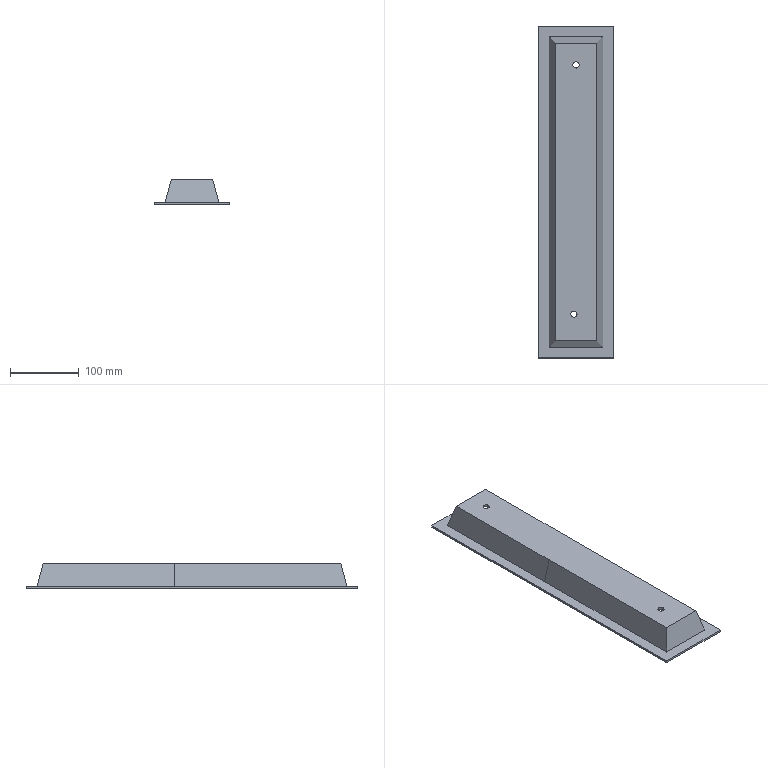Part | NX | features BREP 1 | 1 solid | 28 faces | box 110 x 481.5 x 37.13 mm | volume 237895 mm3 | plane 20 | cylinder 8 | commonest cylinder face diameters 9 x8
STEP:
#1=CARTESIAN_POINT('',(1766.215,0.,67.005));
#2=VERTEX_POINT('',#1);
#3=CARTESIAN_POINT('',(1757.07,0.,101.135));
#4=VERTEX_POINT('',#3);
#5=CARTESIAN_POINT('',(1766.215,0.,67.005));
#6=CARTESIAN_POINT('',(1757.07,0.,101.135));
#7=B_SPLINE_CURVE_WITH_KNOTS('',1,(#5,#6),.UNSPECIFIED.,.F.,.F.,(2,2),(20.364,55.698),.UNSPECIFIED.);
#8=EDGE_CURVE('',#2,#4,#7,.T.);
#9=ORIENTED_EDGE('',*,*,#8,.F.);
#10=CARTESIAN_POINT('',(1766.215,-247.843,67.005));
#11=VERTEX_POINT('',#10);
#12=CARTESIAN_POINT('',(1766.215,-123.922,67.005));
#13=DIRECTION('',(0.,1.,0.));
#14=VECTOR('',#13,1000.);
#15=LINE('',#12,#14);
#16=EDGE_CURVE('',#11,#2,#15,.T.);
#17=ORIENTED_EDGE('',*,*,#16,.F.);
#18=CARTESIAN_POINT('',(1757.07,-238.698,101.135));
#19=VERTEX_POINT('',#18);
#20=CARTESIAN_POINT('',(1761.643,-243.271,84.07));
#21=DIRECTION('',(-0.2506,0.2506,0.9351));
#22=VECTOR('',#21,1000.);
#23=LINE('',#20,#22);
#24=EDGE_CURVE('',#11,#19,#23,.T.);
#25=ORIENTED_EDGE('',*,*,#24,.T.);
#26=CARTESIAN_POINT('',(1757.07,-119.349,101.135));
#27=DIRECTION('',(0.,1.,0.));
#28=VECTOR('',#27,1000.);
#29=LINE('',#26,#28);
#30=EDGE_CURVE('',#19,#4,#29,.T.);
#31=ORIENTED_EDGE('',*,*,#30,.T.);
#32=EDGE_LOOP('',(#9,#17,#25,#31));
#33=FACE_BOUND('',#32,.T.);
#34=CARTESIAN_POINT('',(1761.643,-123.922,84.07));
#35=DIRECTION('',(0.9659,0.,0.2588));
#36=DIRECTION('',(0.2588,0.,-0.9659));
#37=AXIS2_PLACEMENT_3D('',#34,#35,#36);
#38=PLANE('',#37);
#39=ADVANCED_FACE('',(#33),#38,.F.);
#40=ORIENTED_EDGE('',*,*,#24,.F.);
#41=CARTESIAN_POINT('',(1692.529,-247.843,67.005));
#42=VERTEX_POINT('',#41);
#43=CARTESIAN_POINT('',(1729.372,-247.843,67.005));
#44=DIRECTION('',(1.,0.,0.));
#45=VECTOR('',#44,1000.);
#46=LINE('',#43,#45);
#47=EDGE_CURVE('',#42,#11,#46,.T.);
#48=ORIENTED_EDGE('',*,*,#47,.F.);
#49=CARTESIAN_POINT('',(1701.674,-238.698,101.135));
#50=VERTEX_POINT('',#49);
#51=CARTESIAN_POINT('',(1692.529,-247.843,67.005));
#52=CARTESIAN_POINT('',(1701.674,-238.698,101.135));
#53=B_SPLINE_CURVE_WITH_KNOTS('',1,(#51,#52),.UNSPECIFIED.,.F.,.F.,(2,2),(-18.249,18.249),.UNSPECIFIED.);
#54=EDGE_CURVE('',#42,#50,#53,.T.);
#55=ORIENTED_EDGE('',*,*,#54,.T.);
#56=CARTESIAN_POINT('',(1729.372,-238.698,101.135));
#57=DIRECTION('',(1.,0.,0.));
#58=VECTOR('',#57,1000.);
#59=LINE('',#56,#58);
#60=EDGE_CURVE('',#50,#19,#59,.T.);
#61=ORIENTED_EDGE('',*,*,#60,.T.);
#62=EDGE_LOOP('',(#40,#48,#55,#61));
#63=FACE_BOUND('',#62,.T.);
#64=CARTESIAN_POINT('',(1692.529,-247.843,67.005));
#65=DIRECTION('',(0.,-0.9659,0.2588));
#66=DIRECTION('',(1.,0.,0.));
#67=AXIS2_PLACEMENT_3D('',#64,#65,#66);
#68=PLANE('',#67);
#69=ADVANCED_FACE('',(#63),#68,.F.);
#70=CARTESIAN_POINT('',(1701.674,0.,101.135));
#71=VERTEX_POINT('',#70);
#72=CARTESIAN_POINT('',(1701.674,-119.349,101.135));
#73=DIRECTION('',(0.,-1.,0.));
#74=VECTOR('',#73,1000.);
#75=LINE('',#72,#74);
#76=EDGE_CURVE('',#71,#50,#75,.T.);
#77=ORIENTED_EDGE('',*,*,#76,.T.);
#78=ORIENTED_EDGE('',*,*,#54,.F.);
#79=CARTESIAN_POINT('',(1692.529,0.,67.005));
#80=VERTEX_POINT('',#79);
#81=CARTESIAN_POINT('',(1692.529,-123.922,67.005));
#82=DIRECTION('',(0.,1.,0.));
#83=VECTOR('',#82,1000.);
#84=LINE('',#81,#83);
#85=EDGE_CURVE('',#42,#80,#84,.T.);
#86=ORIENTED_EDGE('',*,*,#85,.T.);
#87=CARTESIAN_POINT('',(1692.529,0.,67.005));
#88=CARTESIAN_POINT('',(1701.674,0.,101.135));
#89=B_SPLINE_CURVE_WITH_KNOTS('',1,(#87,#88),.UNSPECIFIED.,.F.,.F.,(2,2),(20.364,55.698),.UNSPECIFIED.);
#90=EDGE_CURVE('',#80,#71,#89,.T.);
#91=ORIENTED_EDGE('',*,*,#90,.T.);
#92=EDGE_LOOP('',(#77,#78,#86,#91));
#93=FACE_BOUND('',#92,.T.);
#94=CARTESIAN_POINT('',(1697.102,-123.922,84.07));
#95=DIRECTION('',(-0.9659,0.,0.2588));
#96=DIRECTION('',(0.2588,0.,0.9659));
#97=AXIS2_PLACEMENT_3D('',#94,#95,#96);
#98=PLANE('',#97);
#99=ADVANCED_FACE('',(#93),#98,.F.);
#100=CARTESIAN_POINT('',(1692.529,197.343,67.005));
#101=VERTEX_POINT('',#100);
#102=CARTESIAN_POINT('',(1692.529,98.672,67.005));
#103=DIRECTION('',(0.,1.,0.));
#104=VECTOR('',#103,1000.);
#105=LINE('',#102,#104);
#106=EDGE_CURVE('',#80,#101,#105,.T.);
#107=ORIENTED_EDGE('',*,*,#106,.T.);
#108=CARTESIAN_POINT('',(1701.674,188.198,101.135));
#109=VERTEX_POINT('',#108);
#110=CARTESIAN_POINT('',(1692.529,197.343,67.005));
#111=CARTESIAN_POINT('',(1695.577,194.295,78.381));
#112=CARTESIAN_POINT('',(1698.626,191.246,89.758));
#113=CARTESIAN_POINT('',(1701.674,188.198,101.135));
#114=B_SPLINE_CURVE_WITH_KNOTS('',3,(#110,#111,#112,#113),.UNSPECIFIED.,.F.,.F.,(4,4),(-18.249,18.249),.UNSPECIFIED.);
#115=EDGE_CURVE('',#101,#109,#114,.T.);
#116=ORIENTED_EDGE('',*,*,#115,.T.);
#117=CARTESIAN_POINT('',(1701.674,94.099,101.135));
#118=DIRECTION('',(0.,-1.,0.));
#119=VECTOR('',#118,1000.);
#120=LINE('',#117,#119);
#121=EDGE_CURVE('',#109,#71,#120,.T.);
#122=ORIENTED_EDGE('',*,*,#121,.T.);
#123=ORIENTED_EDGE('',*,*,#90,.F.);
#124=EDGE_LOOP('',(#107,#116,#122,#123));
#125=FACE_BOUND('',#124,.T.);
#126=CARTESIAN_POINT('',(1697.102,98.672,84.07));
#127=DIRECTION('',(-0.9659,0.,0.2588));
#128=DIRECTION('',(0.2588,0.,0.9659));
#129=AXIS2_PLACEMENT_3D('',#126,#127,#128);
#130=PLANE('',#129);
#131=ADVANCED_FACE('',(#125),#130,.F.);
#132=ORIENTED_EDGE('',*,*,#115,.F.);
#133=CARTESIAN_POINT('',(1766.215,197.343,67.005));
#134=VERTEX_POINT('',#133);
#135=CARTESIAN_POINT('',(1729.372,197.343,67.005));
#136=DIRECTION('',(1.,0.,0.));
#137=VECTOR('',#136,1000.);
#138=LINE('',#135,#137);
#139=EDGE_CURVE('',#101,#134,#138,.T.);
#140=ORIENTED_EDGE('',*,*,#139,.T.);
#141=CARTESIAN_POINT('',(1757.07,188.198,101.135));
#142=VERTEX_POINT('',#141);
#143=CARTESIAN_POINT('',(1766.215,197.343,67.005));
#144=CARTESIAN_POINT('',(1757.07,188.198,101.135));
#145=B_SPLINE_CURVE_WITH_KNOTS('',1,(#143,#144),.UNSPECIFIED.,.F.,.F.,(2,2),(-18.249,18.249),.UNSPECIFIED.);
#146=EDGE_CURVE('',#134,#142,#145,.T.);
#147=ORIENTED_EDGE('',*,*,#146,.T.);
#148=CARTESIAN_POINT('',(1729.372,188.198,101.135));
#149=DIRECTION('',(-1.,0.,0.));
#150=VECTOR('',#149,1000.);
#151=LINE('',#148,#150);
#152=EDGE_CURVE('',#142,#109,#151,.T.);
#153=ORIENTED_EDGE('',*,*,#152,.T.);
#154=EDGE_LOOP('',(#132,#140,#147,#153));
#155=FACE_BOUND('',#154,.T.);
#156=CARTESIAN_POINT('',(1729.372,192.771,84.07));
#157=DIRECTION('',(0.,0.9659,0.2588));
#158=DIRECTION('',(0.,-0.2588,0.9659));
#159=AXIS2_PLACEMENT_3D('',#156,#157,#158);
#160=PLANE('',#159);
#161=ADVANCED_FACE('',(#155),#160,.F.);
#162=CARTESIAN_POINT('',(1757.07,94.099,101.135));
#163=DIRECTION('',(0.,1.,0.));
#164=VECTOR('',#163,1000.);
#165=LINE('',#162,#164);
#166=EDGE_CURVE('',#4,#142,#165,.T.);
#167=ORIENTED_EDGE('',*,*,#166,.T.);
#168=ORIENTED_EDGE('',*,*,#146,.F.);
#169=CARTESIAN_POINT('',(1766.215,98.672,67.005));
#170=DIRECTION('',(0.,1.,0.));
#171=VECTOR('',#170,1000.);
#172=LINE('',#169,#171);
#173=EDGE_CURVE('',#2,#134,#172,.T.);
#174=ORIENTED_EDGE('',*,*,#173,.F.);
#175=ORIENTED_EDGE('',*,*,#8,.T.);
#176=EDGE_LOOP('',(#167,#168,#174,#175));
#177=FACE_BOUND('',#176,.T.);
#178=CARTESIAN_POINT('',(1761.643,98.672,84.07));
#179=DIRECTION('',(0.9659,0.,0.2588));
#180=DIRECTION('',(0.2588,0.,-0.9659));
#181=AXIS2_PLACEMENT_3D('',#178,#179,#180);
#182=PLANE('',#181);
#183=ADVANCED_FACE('',(#177),#182,.F.);
#184=CARTESIAN_POINT('',(1730.872,-202.5,101.135));
#185=VERTEX_POINT('',#184);
#186=CARTESIAN_POINT('',(1726.372,-198.,101.135));
#187=VERTEX_POINT('',#186);
#188=CARTESIAN_POINT('',(1726.372,-202.5,101.135));
#189=DIRECTION('',(0.,0.,1.));
#190=DIRECTION('',(1.,0.,0.));
#191=AXIS2_PLACEMENT_3D('',#188,#189,#190);
#192=CIRCLE('',#191,4.5);
#193=EDGE_CURVE('',#185,#187,#192,.T.);
#194=ORIENTED_EDGE('',*,*,#193,.T.);
#195=CARTESIAN_POINT('',(1721.872,-202.5,101.135));
#196=VERTEX_POINT('',#195);
#197=CARTESIAN_POINT('',(1726.372,-202.5,101.135));
#198=DIRECTION('',(0.,0.,1.));
#199=DIRECTION('',(1.,0.,0.));
#200=AXIS2_PLACEMENT_3D('',#197,#198,#199);
#201=CIRCLE('',#200,4.5);
#202=EDGE_CURVE('',#187,#196,#201,.T.);
#203=ORIENTED_EDGE('',*,*,#202,.T.);
#204=CARTESIAN_POINT('',(1726.372,-207.,101.135));
#205=VERTEX_POINT('',#204);
#206=CARTESIAN_POINT('',(1726.372,-202.5,101.135));
#207=DIRECTION('',(0.,0.,1.));
#208=DIRECTION('',(1.,0.,0.));
#209=AXIS2_PLACEMENT_3D('',#206,#207,#208);
#210=CIRCLE('',#209,4.5);
#211=EDGE_CURVE('',#196,#205,#210,.T.);
#212=ORIENTED_EDGE('',*,*,#211,.T.);
#213=CARTESIAN_POINT('',(1726.372,-202.5,101.135));
#214=DIRECTION('',(0.,0.,1.));
#215=DIRECTION('',(1.,0.,0.));
#216=AXIS2_PLACEMENT_3D('',#213,#214,#215);
#217=CIRCLE('',#216,4.5);
#218=EDGE_CURVE('',#205,#185,#217,.T.);
#219=ORIENTED_EDGE('',*,*,#218,.T.);
#220=EDGE_LOOP('',(#194,#203,#212,#219));
#221=FACE_BOUND('',#220,.T.);
#222=CARTESIAN_POINT('',(1733.872,159.,101.135));
#223=VERTEX_POINT('',#222);
#224=CARTESIAN_POINT('',(1729.372,163.5,101.135));
#225=VERTEX_POINT('',#224);
#226=CARTESIAN_POINT('',(1729.372,159.,101.135));
#227=DIRECTION('',(0.,0.,1.));
#228=DIRECTION('',(1.,0.,0.));
#229=AXIS2_PLACEMENT_3D('',#226,#227,#228);
#230=CIRCLE('',#229,4.5);
#231=EDGE_CURVE('',#223,#225,#230,.T.);
#232=ORIENTED_EDGE('',*,*,#231,.T.);
#233=CARTESIAN_POINT('',(1724.872,159.,101.135));
#234=VERTEX_POINT('',#233);
#235=CARTESIAN_POINT('',(1729.372,159.,101.135));
#236=DIRECTION('',(0.,0.,1.));
#237=DIRECTION('',(1.,0.,0.));
#238=AXIS2_PLACEMENT_3D('',#235,#236,#237);
#239=CIRCLE('',#238,4.5);
#240=EDGE_CURVE('',#225,#234,#239,.T.);
#241=ORIENTED_EDGE('',*,*,#240,.T.);
#242=CARTESIAN_POINT('',(1729.372,154.5,101.135));
#243=VERTEX_POINT('',#242);
#244=CARTESIAN_POINT('',(1729.372,159.,101.135));
#245=DIRECTION('',(0.,0.,1.));
#246=DIRECTION('',(1.,0.,0.));
#247=AXIS2_PLACEMENT_3D('',#244,#245,#246);
#248=CIRCLE('',#247,4.5);
#249=EDGE_CURVE('',#234,#243,#248,.T.);
#250=ORIENTED_EDGE('',*,*,#249,.T.);
#251=CARTESIAN_POINT('',(1729.372,159.,101.135));
#252=DIRECTION('',(0.,0.,1.));
#253=DIRECTION('',(1.,0.,0.));
#254=AXIS2_PLACEMENT_3D('',#251,#252,#253);
#255=CIRCLE('',#254,4.5);
#256=EDGE_CURVE('',#243,#223,#255,.T.);
#257=ORIENTED_EDGE('',*,*,#256,.T.);
#258=EDGE_LOOP('',(#232,#241,#250,#257));
#259=FACE_BOUND('',#258,.T.);
#260=ORIENTED_EDGE('',*,*,#166,.F.);
#261=ORIENTED_EDGE('',*,*,#30,.F.);
#262=ORIENTED_EDGE('',*,*,#60,.F.);
#263=ORIENTED_EDGE('',*,*,#76,.F.);
#264=ORIENTED_EDGE('',*,*,#121,.F.);
#265=ORIENTED_EDGE('',*,*,#152,.F.);
#266=EDGE_LOOP('',(#260,#261,#262,#263,#264,#265));
#267=FACE_BOUND('',#266,.T.);
#268=CARTESIAN_POINT('',(450.,0.,101.135));
#269=DIRECTION('',(0.,0.,1.));
#270=DIRECTION('',(1.,0.,0.));
#271=AXIS2_PLACEMENT_3D('',#268,#269,#270);
#272=PLANE('',#271);
#273=ADVANCED_FACE('',(#221,#259,#267),#272,.F.);
#274=ORIENTED_EDGE('',*,*,#173,.T.);
#275=ORIENTED_EDGE('',*,*,#139,.F.);
#276=ORIENTED_EDGE('',*,*,#106,.F.);
#277=ORIENTED_EDGE('',*,*,#85,.F.);
#278=ORIENTED_EDGE('',*,*,#47,.T.);
#279=ORIENTED_EDGE('',*,*,#16,.T.);
#280=EDGE_LOOP('',(#274,#275,#276,#277,#278,#279));
#281=FACE_BOUND('',#280,.T.);
#282=CARTESIAN_POINT('',(1674.372,215.5,67.005));
#283=VERTEX_POINT('',#282);
#284=CARTESIAN_POINT('',(1784.372,215.5,67.005));
#285=VERTEX_POINT('',#284);
#286=CARTESIAN_POINT('',(1729.372,215.5,67.005));
#287=DIRECTION('',(1.,0.,0.));
#288=VECTOR('',#287,1000.);
#289=LINE('',#286,#288);
#290=EDGE_CURVE('',#283,#285,#289,.T.);
#291=ORIENTED_EDGE('',*,*,#290,.T.);
#292=CARTESIAN_POINT('',(1784.372,-266.,67.005));
#293=VERTEX_POINT('',#292);
#294=CARTESIAN_POINT('',(1784.372,-25.25,67.005));
#295=DIRECTION('',(0.,1.,0.));
#296=VECTOR('',#295,1000.);
#297=LINE('',#294,#296);
#298=EDGE_CURVE('',#293,#285,#297,.T.);
#299=ORIENTED_EDGE('',*,*,#298,.F.);
#300=CARTESIAN_POINT('',(1674.372,-266.,67.005));
#301=VERTEX_POINT('',#300);
#302=CARTESIAN_POINT('',(1729.372,-266.,67.005));
#303=DIRECTION('',(1.,0.,0.));
#304=VECTOR('',#303,1000.);
#305=LINE('',#302,#304);
#306=EDGE_CURVE('',#301,#293,#305,.T.);
#307=ORIENTED_EDGE('',*,*,#306,.F.);
#308=CARTESIAN_POINT('',(1674.372,-25.25,67.005));
#309=DIRECTION('',(0.,1.,0.));
#310=VECTOR('',#309,1000.);
#311=LINE('',#308,#310);
#312=EDGE_CURVE('',#301,#283,#311,.T.);
#313=ORIENTED_EDGE('',*,*,#312,.T.);
#314=EDGE_LOOP('',(#291,#299,#307,#313));
#315=FACE_BOUND('',#314,.T.);
#316=CARTESIAN_POINT('',(450.,0.,67.005));
#317=DIRECTION('',(0.,0.,1.));
#318=DIRECTION('',(1.,0.,0.));
#319=AXIS2_PLACEMENT_3D('',#316,#317,#318);
#320=PLANE('',#319);
#321=ADVANCED_FACE('',(#281,#315),#320,.F.);
#322=ORIENTED_EDGE('',*,*,#193,.F.);
#323=CARTESIAN_POINT('',(1730.872,-202.5,104.135));
#324=VERTEX_POINT('',#323);
#325=CARTESIAN_POINT('',(1730.872,-202.5,104.135));
#326=DIRECTION('',(0.,0.,1.));
#327=VECTOR('',#326,1000.);
#328=LINE('',#325,#327);
#329=EDGE_CURVE('',#185,#324,#328,.T.);
#330=ORIENTED_EDGE('',*,*,#329,.T.);
#331=CARTESIAN_POINT('',(1726.372,-198.,104.135));
#332=VERTEX_POINT('',#331);
#333=CARTESIAN_POINT('',(1726.372,-202.5,104.135));
#334=DIRECTION('',(0.,0.,1.));
#335=DIRECTION('',(1.,0.,0.));
#336=AXIS2_PLACEMENT_3D('',#333,#334,#335);
#337=CIRCLE('',#336,4.5);
#338=EDGE_CURVE('',#324,#332,#337,.T.);
#339=ORIENTED_EDGE('',*,*,#338,.T.);
#340=CARTESIAN_POINT('',(1726.372,-198.,104.135));
#341=DIRECTION('',(0.,0.,1.));
#342=VECTOR('',#341,1000.);
#343=LINE('',#340,#342);
#344=EDGE_CURVE('',#187,#332,#343,.T.);
#345=ORIENTED_EDGE('',*,*,#344,.F.);
#346=EDGE_LOOP('',(#322,#330,#339,#345));
#347=FACE_BOUND('',#346,.T.);
#348=CARTESIAN_POINT('',(1726.372,-202.5,104.135));
#349=DIRECTION('',(0.,0.,1.));
#350=DIRECTION('',(0.,-1.,0.));
#351=AXIS2_PLACEMENT_3D('',#348,#349,#350);
#352=CYLINDRICAL_SURFACE('',#351,4.5);
#353=ADVANCED_FACE('',(#347),#352,.F.);
#354=CARTESIAN_POINT('',(1721.872,-202.5,104.135));
#355=VERTEX_POINT('',#354);
#356=CARTESIAN_POINT('',(1726.372,-202.5,104.135));
#357=DIRECTION('',(0.,0.,1.));
#358=DIRECTION('',(1.,0.,0.));
#359=AXIS2_PLACEMENT_3D('',#356,#357,#358);
#360=CIRCLE('',#359,4.5);
#361=EDGE_CURVE('',#332,#355,#360,.T.);
#362=ORIENTED_EDGE('',*,*,#361,.T.);
#363=CARTESIAN_POINT('',(1721.872,-202.5,104.135));
#364=DIRECTION('',(0.,0.,1.));
#365=VECTOR('',#364,1000.);
#366=LINE('',#363,#365);
#367=EDGE_CURVE('',#196,#355,#366,.T.);
#368=ORIENTED_EDGE('',*,*,#367,.F.);
#369=ORIENTED_EDGE('',*,*,#202,.F.);
#370=ORIENTED_EDGE('',*,*,#344,.T.);
#371=EDGE_LOOP('',(#362,#368,#369,#370));
#372=FACE_BOUND('',#371,.T.);
#373=CARTESIAN_POINT('',(1726.372,-202.5,104.135));
#374=DIRECTION('',(0.,0.,1.));
#375=DIRECTION('',(0.,1.,0.));
#376=AXIS2_PLACEMENT_3D('',#373,#374,#375);
#377=CYLINDRICAL_SURFACE('',#376,4.5);
#378=ADVANCED_FACE('',(#372),#377,.F.);
#379=ORIENTED_EDGE('',*,*,#211,.F.);
#380=ORIENTED_EDGE('',*,*,#367,.T.);
#381=CARTESIAN_POINT('',(1726.372,-207.,104.135));
#382=VERTEX_POINT('',#381);
#383=CARTESIAN_POINT('',(1726.372,-202.5,104.135));
#384=DIRECTION('',(0.,0.,1.));
#385=DIRECTION('',(1.,0.,0.));
#386=AXIS2_PLACEMENT_3D('',#383,#384,#385);
#387=CIRCLE('',#386,4.5);
#388=EDGE_CURVE('',#355,#382,#387,.T.);
#389=ORIENTED_EDGE('',*,*,#388,.T.);
#390=CARTESIAN_POINT('',(1726.372,-207.,104.135));
#391=DIRECTION('',(0.,0.,1.));
#392=VECTOR('',#391,1000.);
#393=LINE('',#390,#392);
#394=EDGE_CURVE('',#205,#382,#393,.T.);
#395=ORIENTED_EDGE('',*,*,#394,.F.);
#396=EDGE_LOOP('',(#379,#380,#389,#395));
#397=FACE_BOUND('',#396,.T.);
#398=CARTESIAN_POINT('',(1726.372,-202.5,104.135));
#399=DIRECTION('',(0.,0.,1.));
#400=DIRECTION('',(0.,1.,0.));
#401=AXIS2_PLACEMENT_3D('',#398,#399,#400);
#402=CYLINDRICAL_SURFACE('',#401,4.5);
#403=ADVANCED_FACE('',(#397),#402,.F.);
#404=CARTESIAN_POINT('',(1726.372,-202.5,104.135));
#405=DIRECTION('',(0.,0.,1.));
#406=DIRECTION('',(1.,0.,0.));
#407=AXIS2_PLACEMENT_3D('',#404,#405,#406);
#408=CIRCLE('',#407,4.5);
#409=EDGE_CURVE('',#382,#324,#408,.T.);
#410=ORIENTED_EDGE('',*,*,#409,.T.);
#411=ORIENTED_EDGE('',*,*,#329,.F.);
#412=ORIENTED_EDGE('',*,*,#218,.F.);
#413=ORIENTED_EDGE('',*,*,#394,.T.);
#414=EDGE_LOOP('',(#410,#411,#412,#413));
#415=FACE_BOUND('',#414,.T.);
#416=CARTESIAN_POINT('',(1726.372,-202.5,104.135));
#417=DIRECTION('',(0.,0.,1.));
#418=DIRECTION('',(0.,-1.,0.));
#419=AXIS2_PLACEMENT_3D('',#416,#417,#418);
#420=CYLINDRICAL_SURFACE('',#419,4.5);
#421=ADVANCED_FACE('',(#415),#420,.F.);
#422=ORIENTED_EDGE('',*,*,#231,.F.);
#423=CARTESIAN_POINT('',(1733.872,159.,104.135));
#424=VERTEX_POINT('',#423);
#425=CARTESIAN_POINT('',(1733.872,159.,104.135));
#426=DIRECTION('',(0.,0.,1.));
#427=VECTOR('',#426,1000.);
#428=LINE('',#425,#427);
#429=EDGE_CURVE('',#223,#424,#428,.T.);
#430=ORIENTED_EDGE('',*,*,#429,.T.);
#431=CARTESIAN_POINT('',(1729.372,163.5,104.135));
#432=VERTEX_POINT('',#431);
#433=CARTESIAN_POINT('',(1729.372,159.,104.135));
#434=DIRECTION('',(0.,0.,1.));
#435=DIRECTION('',(1.,0.,0.));
#436=AXIS2_PLACEMENT_3D('',#433,#434,#435);
#437=CIRCLE('',#436,4.5);
#438=EDGE_CURVE('',#424,#432,#437,.T.);
#439=ORIENTED_EDGE('',*,*,#438,.T.);
#440=CARTESIAN_POINT('',(1729.372,163.5,104.135));
#441=DIRECTION('',(0.,0.,1.));
#442=VECTOR('',#441,1000.);
#443=LINE('',#440,#442);
#444=EDGE_CURVE('',#225,#432,#443,.T.);
#445=ORIENTED_EDGE('',*,*,#444,.F.);
#446=EDGE_LOOP('',(#422,#430,#439,#445));
#447=FACE_BOUND('',#446,.T.);
#448=CARTESIAN_POINT('',(1729.372,159.,104.135));
#449=DIRECTION('',(0.,0.,1.));
#450=DIRECTION('',(0.,-1.,0.));
#451=AXIS2_PLACEMENT_3D('',#448,#449,#450);
#452=CYLINDRICAL_SURFACE('',#451,4.5);
#453=ADVANCED_FACE('',(#447),#452,.F.);
#454=CARTESIAN_POINT('',(1724.872,159.,104.135));
#455=VERTEX_POINT('',#454);
#456=CARTESIAN_POINT('',(1729.372,159.,104.135));
#457=DIRECTION('',(0.,0.,1.));
#458=DIRECTION('',(1.,0.,0.));
#459=AXIS2_PLACEMENT_3D('',#456,#457,#458);
#460=CIRCLE('',#459,4.5);
#461=EDGE_CURVE('',#432,#455,#460,.T.);
#462=ORIENTED_EDGE('',*,*,#461,.T.);
#463=CARTESIAN_POINT('',(1724.872,159.,104.135));
#464=DIRECTION('',(0.,0.,1.));
#465=VECTOR('',#464,1000.);
#466=LINE('',#463,#465);
#467=EDGE_CURVE('',#234,#455,#466,.T.);
#468=ORIENTED_EDGE('',*,*,#467,.F.);
#469=ORIENTED_EDGE('',*,*,#240,.F.);
#470=ORIENTED_EDGE('',*,*,#444,.T.);
#471=EDGE_LOOP('',(#462,#468,#469,#470));
#472=FACE_BOUND('',#471,.T.);
#473=CARTESIAN_POINT('',(1729.372,159.,104.135));
#474=DIRECTION('',(0.,0.,1.));
#475=DIRECTION('',(0.,1.,0.));
#476=AXIS2_PLACEMENT_3D('',#473,#474,#475);
#477=CYLINDRICAL_SURFACE('',#476,4.5);
#478=ADVANCED_FACE('',(#472),#477,.F.);
#479=ORIENTED_EDGE('',*,*,#249,.F.);
#480=ORIENTED_EDGE('',*,*,#467,.T.);
#481=CARTESIAN_POINT('',(1729.372,154.5,104.135));
#482=VERTEX_POINT('',#481);
#483=CARTESIAN_POINT('',(1729.372,159.,104.135));
#484=DIRECTION('',(0.,0.,1.));
#485=DIRECTION('',(1.,0.,0.));
#486=AXIS2_PLACEMENT_3D('',#483,#484,#485);
#487=CIRCLE('',#486,4.5);
#488=EDGE_CURVE('',#455,#482,#487,.T.);
#489=ORIENTED_EDGE('',*,*,#488,.T.);
#490=CARTESIAN_POINT('',(1729.372,154.5,104.135));
#491=DIRECTION('',(0.,0.,1.));
#492=VECTOR('',#491,1000.);
#493=LINE('',#490,#492);
#494=EDGE_CURVE('',#243,#482,#493,.T.);
#495=ORIENTED_EDGE('',*,*,#494,.F.);
#496=EDGE_LOOP('',(#479,#480,#489,#495));
#497=FACE_BOUND('',#496,.T.);
#498=CARTESIAN_POINT('',(1729.372,159.,104.135));
#499=DIRECTION('',(0.,0.,1.));
#500=DIRECTION('',(0.,1.,0.));
#501=AXIS2_PLACEMENT_3D('',#498,#499,#500);
#502=CYLINDRICAL_SURFACE('',#501,4.5);
#503=ADVANCED_FACE('',(#497),#502,.F.);
#504=CARTESIAN_POINT('',(1729.372,159.,104.135));
#505=DIRECTION('',(0.,0.,1.));
#506=DIRECTION('',(1.,0.,0.));
#507=AXIS2_PLACEMENT_3D('',#504,#505,#506);
#508=CIRCLE('',#507,4.5);
#509=EDGE_CURVE('',#482,#424,#508,.T.);
#510=ORIENTED_EDGE('',*,*,#509,.T.);
#511=ORIENTED_EDGE('',*,*,#429,.F.);
#512=ORIENTED_EDGE('',*,*,#256,.F.);
#513=ORIENTED_EDGE('',*,*,#494,.T.);
#514=EDGE_LOOP('',(#510,#511,#512,#513));
#515=FACE_BOUND('',#514,.T.);
#516=CARTESIAN_POINT('',(1729.372,159.,104.135));
#517=DIRECTION('',(0.,0.,1.));
#518=DIRECTION('',(0.,-1.,0.));
#519=AXIS2_PLACEMENT_3D('',#516,#517,#518);
#520=CYLINDRICAL_SURFACE('',#519,4.5);
#521=ADVANCED_FACE('',(#515),#520,.F.);
#522=CARTESIAN_POINT('',(1768.517,0.,70.005));
#523=VERTEX_POINT('',#522);
#524=CARTESIAN_POINT('',(1759.372,0.,104.135));
#525=VERTEX_POINT('',#524);
#526=CARTESIAN_POINT('',(1768.517,0.,70.005));
#527=CARTESIAN_POINT('',(1759.372,0.,104.135));
#528=B_SPLINE_CURVE_WITH_KNOTS('',1,(#526,#527),.UNSPECIFIED.,.F.,.F.,(2,2),(22.666,58.),.UNSPECIFIED.);
#529=EDGE_CURVE('',#523,#525,#528,.T.);
#530=ORIENTED_EDGE('',*,*,#529,.F.);
#531=CARTESIAN_POINT('',(1768.517,199.645,70.005));
#532=VERTEX_POINT('',#531);
#533=CARTESIAN_POINT('',(1768.517,99.823,70.005));
#534=DIRECTION('',(0.,1.,0.));
#535=VECTOR('',#534,1000.);
#536=LINE('',#533,#535);
#537=EDGE_CURVE('',#523,#532,#536,.T.);
#538=ORIENTED_EDGE('',*,*,#537,.T.);
#539=CARTESIAN_POINT('',(1759.372,190.5,104.135));
#540=VERTEX_POINT('',#539);
#541=CARTESIAN_POINT('',(1768.517,199.645,70.005));
#542=CARTESIAN_POINT('',(1759.372,190.5,104.135));
#543=B_SPLINE_CURVE_WITH_KNOTS('',1,(#541,#542),.UNSPECIFIED.,.F.,.F.,(2,2),(-18.249,18.249),.UNSPECIFIED.);
#544=EDGE_CURVE('',#532,#540,#543,.T.);
#545=ORIENTED_EDGE('',*,*,#544,.T.);
#546=CARTESIAN_POINT('',(1759.372,95.25,104.135));
#547=DIRECTION('',(0.,1.,0.));
#548=VECTOR('',#547,1000.);
#549=LINE('',#546,#548);
#550=EDGE_CURVE('',#525,#540,#549,.T.);
#551=ORIENTED_EDGE('',*,*,#550,.F.);
#552=EDGE_LOOP('',(#530,#538,#545,#551));
#553=FACE_BOUND('',#552,.T.);
#554=CARTESIAN_POINT('',(1766.878,-50.5,76.123));
#555=DIRECTION('',(0.9659,0.,0.2588));
#556=DIRECTION('',(0.2588,0.,-0.9659));
#557=AXIS2_PLACEMENT_3D('',#554,#555,#556);
#558=PLANE('',#557);
#559=ADVANCED_FACE('',(#553),#558,.T.);
#560=CARTESIAN_POINT('',(1759.372,-241.,104.135));
#561=VERTEX_POINT('',#560);
#562=CARTESIAN_POINT('',(1759.372,-120.5,104.135));
#563=DIRECTION('',(0.,1.,0.));
#564=VECTOR('',#563,1000.);
#565=LINE('',#562,#564);
#566=EDGE_CURVE('',#561,#525,#565,.T.);
#567=ORIENTED_EDGE('',*,*,#566,.F.);
#568=CARTESIAN_POINT('',(1768.517,-250.145,70.005));
#569=VERTEX_POINT('',#568);
#570=CARTESIAN_POINT('',(1768.517,-250.145,70.005));
#571=CARTESIAN_POINT('',(1759.372,-241.,104.135));
#572=B_SPLINE_CURVE_WITH_KNOTS('',1,(#570,#571),.UNSPECIFIED.,.F.,.F.,(2,2),(-18.249,18.249),.UNSPECIFIED.);
#573=EDGE_CURVE('',#569,#561,#572,.T.);
#574=ORIENTED_EDGE('',*,*,#573,.F.);
#575=CARTESIAN_POINT('',(1768.517,-125.073,70.005));
#576=DIRECTION('',(0.,1.,0.));
#577=VECTOR('',#576,1000.);
#578=LINE('',#575,#577);
#579=EDGE_CURVE('',#569,#523,#578,.T.);
#580=ORIENTED_EDGE('',*,*,#579,.T.);
#581=ORIENTED_EDGE('',*,*,#529,.T.);
#582=EDGE_LOOP('',(#567,#574,#580,#581));
#583=FACE_BOUND('',#582,.T.);
#584=CARTESIAN_POINT('',(1766.878,0.000003927,76.123));
#585=DIRECTION('',(0.9659,0.,0.2588));
#586=DIRECTION('',(0.2588,0.,-0.9659));
#587=AXIS2_PLACEMENT_3D('',#584,#585,#586);
#588=PLANE('',#587);
#589=ADVANCED_FACE('',(#583),#588,.T.);
#590=CARTESIAN_POINT('',(1674.372,215.5,70.005));
#591=VERTEX_POINT('',#590);
#592=CARTESIAN_POINT('',(1784.372,215.5,70.005));
#593=VERTEX_POINT('',#592);
#594=CARTESIAN_POINT('',(1729.372,215.5,70.005));
#595=DIRECTION('',(1.,0.,0.));
#596=VECTOR('',#595,1000.);
#597=LINE('',#594,#596);
#598=EDGE_CURVE('',#591,#593,#597,.T.);
#599=ORIENTED_EDGE('',*,*,#598,.T.);
#600=CARTESIAN_POINT('',(1784.372,215.5,68.505));
#601=DIRECTION('',(0.,0.,-1.));
#602=VECTOR('',#601,1000.);
#603=LINE('',#600,#602);
#604=EDGE_CURVE('',#593,#285,#603,.T.);
#605=ORIENTED_EDGE('',*,*,#604,.T.);
#606=ORIENTED_EDGE('',*,*,#290,.F.);
#607=CARTESIAN_POINT('',(1674.372,215.5,68.505));
#608=DIRECTION('',(0.,0.,-1.));
#609=VECTOR('',#608,1000.);
#610=LINE('',#607,#609);
#611=EDGE_CURVE('',#591,#283,#610,.T.);
#612=ORIENTED_EDGE('',*,*,#611,.F.);
#613=EDGE_LOOP('',(#599,#605,#606,#612));
#614=FACE_BOUND('',#613,.T.);
#615=CARTESIAN_POINT('',(1729.372,215.5,70.005));
#616=DIRECTION('',(0.,1.,0.));
#617=DIRECTION('',(1.,0.,0.));
#618=AXIS2_PLACEMENT_3D('',#615,#616,#617);
#619=PLANE('',#618);
#620=ADVANCED_FACE('',(#614),#619,.T.);
#621=CARTESIAN_POINT('',(1784.372,-266.,70.005));
#622=VERTEX_POINT('',#621);
#623=CARTESIAN_POINT('',(1784.372,-25.25,70.005));
#624=DIRECTION('',(0.,-1.,0.));
#625=VECTOR('',#624,1000.);
#626=LINE('',#623,#625);
#627=EDGE_CURVE('',#593,#622,#626,.T.);
#628=ORIENTED_EDGE('',*,*,#627,.T.);
#629=CARTESIAN_POINT('',(1784.372,-266.,68.505));
#630=DIRECTION('',(0.,0.,-1.));
#631=VECTOR('',#630,1000.);
#632=LINE('',#629,#631);
#633=EDGE_CURVE('',#622,#293,#632,.T.);
#634=ORIENTED_EDGE('',*,*,#633,.T.);
#635=ORIENTED_EDGE('',*,*,#298,.T.);
#636=ORIENTED_EDGE('',*,*,#604,.F.);
#637=EDGE_LOOP('',(#628,#634,#635,#636));
#638=FACE_BOUND('',#637,.T.);
#639=CARTESIAN_POINT('',(1784.372,-25.25,70.005));
#640=DIRECTION('',(-1.,0.,0.));
#641=DIRECTION('',(0.,0.,-1.));
#642=AXIS2_PLACEMENT_3D('',#639,#640,#641);
#643=PLANE('',#642);
#644=ADVANCED_FACE('',(#638),#643,.F.);
#645=CARTESIAN_POINT('',(1674.372,-266.,70.005));
#646=VERTEX_POINT('',#645);
#647=CARTESIAN_POINT('',(1729.372,-266.,70.005));
#648=DIRECTION('',(1.,0.,0.));
#649=VECTOR('',#648,1000.);
#650=LINE('',#647,#649);
#651=EDGE_CURVE('',#646,#622,#650,.T.);
#652=ORIENTED_EDGE('',*,*,#651,.F.);
#653=CARTESIAN_POINT('',(1674.372,-266.,68.505));
#654=DIRECTION('',(0.,0.,-1.));
#655=VECTOR('',#654,1000.);
#656=LINE('',#653,#655);
#657=EDGE_CURVE('',#646,#301,#656,.T.);
#658=ORIENTED_EDGE('',*,*,#657,.T.);
#659=ORIENTED_EDGE('',*,*,#306,.T.);
#660=ORIENTED_EDGE('',*,*,#633,.F.);
#661=EDGE_LOOP('',(#652,#658,#659,#660));
#662=FACE_BOUND('',#661,.T.);
#663=CARTESIAN_POINT('',(1729.372,-266.,70.005));
#664=DIRECTION('',(0.,1.,0.));
#665=DIRECTION('',(1.,0.,0.));
#666=AXIS2_PLACEMENT_3D('',#663,#664,#665);
#667=PLANE('',#666);
#668=ADVANCED_FACE('',(#662),#667,.F.);
#669=ORIENTED_EDGE('',*,*,#611,.T.);
#670=ORIENTED_EDGE('',*,*,#312,.F.);
#671=ORIENTED_EDGE('',*,*,#657,.F.);
#672=CARTESIAN_POINT('',(1674.372,-25.25,70.005));
#673=DIRECTION('',(0.,1.,0.));
#674=VECTOR('',#673,1000.);
#675=LINE('',#672,#674);
#676=EDGE_CURVE('',#646,#591,#675,.T.);
#677=ORIENTED_EDGE('',*,*,#676,.T.);
#678=EDGE_LOOP('',(#669,#670,#671,#677));
#679=FACE_BOUND('',#678,.T.);
#680=CARTESIAN_POINT('',(1674.372,-25.25,70.005));
#681=DIRECTION('',(1.,0.,0.));
#682=DIRECTION('',(0.,0.,-1.));
#683=AXIS2_PLACEMENT_3D('',#680,#681,#682);
#684=PLANE('',#683);
#685=ADVANCED_FACE('',(#679),#684,.F.);
#686=CARTESIAN_POINT('',(1699.372,190.5,104.135));
#687=VERTEX_POINT('',#686);
#688=CARTESIAN_POINT('',(1729.372,190.5,104.135));
#689=DIRECTION('',(-1.,0.,0.));
#690=VECTOR('',#689,1000.);
#691=LINE('',#688,#690);
#692=EDGE_CURVE('',#540,#687,#691,.T.);
#693=ORIENTED_EDGE('',*,*,#692,.F.);
#694=ORIENTED_EDGE('',*,*,#544,.F.);
#695=CARTESIAN_POINT('',(1690.227,199.645,70.005));
#696=VERTEX_POINT('',#695);
#697=CARTESIAN_POINT('',(1729.372,199.645,70.005));
#698=DIRECTION('',(-1.,0.,0.));
#699=VECTOR('',#698,1000.);
#700=LINE('',#697,#699);
#701=EDGE_CURVE('',#532,#696,#700,.T.);
#702=ORIENTED_EDGE('',*,*,#701,.T.);
#703=CARTESIAN_POINT('',(1690.227,199.645,70.005));
#704=CARTESIAN_POINT('',(1699.372,190.5,104.135));
#705=B_SPLINE_CURVE_WITH_KNOTS('',1,(#703,#704),.UNSPECIFIED.,.F.,.F.,(2,2),(-18.249,18.249),.UNSPECIFIED.);
#706=EDGE_CURVE('',#696,#687,#705,.T.);
#707=ORIENTED_EDGE('',*,*,#706,.T.);
#708=EDGE_LOOP('',(#693,#694,#702,#707));
#709=FACE_BOUND('',#708,.T.);
#710=CARTESIAN_POINT('',(1729.372,198.006,76.123));
#711=DIRECTION('',(0.,0.9659,0.2588));
#712=DIRECTION('',(0.,-0.2588,0.9659));
#713=AXIS2_PLACEMENT_3D('',#710,#711,#712);
#714=PLANE('',#713);
#715=ADVANCED_FACE('',(#709),#714,.T.);
#716=ORIENTED_EDGE('',*,*,#409,.F.);
#717=ORIENTED_EDGE('',*,*,#388,.F.);
#718=ORIENTED_EDGE('',*,*,#361,.F.);
#719=ORIENTED_EDGE('',*,*,#338,.F.);
#720=EDGE_LOOP('',(#716,#717,#718,#719));
#721=FACE_BOUND('',#720,.T.);
#722=ORIENTED_EDGE('',*,*,#509,.F.);
#723=ORIENTED_EDGE('',*,*,#488,.F.);
#724=ORIENTED_EDGE('',*,*,#461,.F.);
#725=ORIENTED_EDGE('',*,*,#438,.F.);
#726=EDGE_LOOP('',(#722,#723,#724,#725));
#727=FACE_BOUND('',#726,.T.);
#728=ORIENTED_EDGE('',*,*,#566,.T.);
#729=ORIENTED_EDGE('',*,*,#550,.T.);
#730=ORIENTED_EDGE('',*,*,#692,.T.);
#731=CARTESIAN_POINT('',(1699.372,0.000000128,104.135));
#732=VERTEX_POINT('',#731);
#733=CARTESIAN_POINT('',(1699.372,190.5,104.135));
#734=CARTESIAN_POINT('',(1699.372,152.4,104.135));
#735=CARTESIAN_POINT('',(1699.372,114.3,104.135));
#736=CARTESIAN_POINT('',(1699.372,76.2,104.135));
#737=CARTESIAN_POINT('',(1699.372,38.1,104.135));
#738=CARTESIAN_POINT('',(1699.372,0.000000385,104.135));
#739=B_SPLINE_CURVE_WITH_KNOTS('',5,(#733,#734,#735,#736,#737,#738),.UNSPECIFIED.,.F.,.F.,(6,6),(30.023,220.523),.UNSPECIFIED.);
#740=EDGE_CURVE('',#687,#732,#739,.T.);
#741=ORIENTED_EDGE('',*,*,#740,.T.);
#742=CARTESIAN_POINT('',(1699.372,-241.,104.135));
#743=VERTEX_POINT('',#742);
#744=CARTESIAN_POINT('',(1699.372,0.,104.135));
#745=CARTESIAN_POINT('',(1699.372,-48.2,104.135));
#746=CARTESIAN_POINT('',(1699.372,-96.4,104.135));
#747=CARTESIAN_POINT('',(1699.372,-144.6,104.135));
#748=CARTESIAN_POINT('',(1699.372,-192.8,104.135));
#749=CARTESIAN_POINT('',(1699.372,-241.,104.135));
#750=B_SPLINE_CURVE_WITH_KNOTS('',5,(#744,#745,#746,#747,#748,#749),.UNSPECIFIED.,.F.,.F.,(6,6),(271.023,512.023),.UNSPECIFIED.);
#751=EDGE_CURVE('',#732,#743,#750,.T.);
#752=ORIENTED_EDGE('',*,*,#751,.T.);
#753=CARTESIAN_POINT('',(1699.372,-241.,104.135));
#754=CARTESIAN_POINT('',(1711.372,-241.,104.135));
#755=CARTESIAN_POINT('',(1723.372,-241.,104.135));
#756=CARTESIAN_POINT('',(1735.372,-241.,104.135));
#757=CARTESIAN_POINT('',(1747.372,-241.,104.135));
#758=CARTESIAN_POINT('',(1759.372,-241.,104.135));
#759=B_SPLINE_CURVE_WITH_KNOTS('',5,(#753,#754,#755,#756,#757,#758),.UNSPECIFIED.,.F.,.F.,(6,6),(30.023,90.023),.UNSPECIFIED.);
#760=EDGE_CURVE('',#743,#561,#759,.T.);
#761=ORIENTED_EDGE('',*,*,#760,.T.);
#762=EDGE_LOOP('',(#728,#729,#730,#741,#752,#761));
#763=FACE_BOUND('',#762,.T.);
#764=CARTESIAN_POINT('',(450.,0.,104.135));
#765=DIRECTION('',(0.,0.,1.));
#766=DIRECTION('',(1.,0.,0.));
#767=AXIS2_PLACEMENT_3D('',#764,#765,#766);
#768=PLANE('',#767);
#769=ADVANCED_FACE('',(#721,#727,#763),#768,.T.);
#770=ORIENTED_EDGE('',*,*,#760,.F.);
#771=CARTESIAN_POINT('',(1690.227,-250.145,70.005));
#772=VERTEX_POINT('',#771);
#773=CARTESIAN_POINT('',(1690.227,-250.145,70.005));
#774=CARTESIAN_POINT('',(1699.372,-241.,104.135));
#775=B_SPLINE_CURVE_WITH_KNOTS('',1,(#773,#774),.UNSPECIFIED.,.F.,.F.,(2,2),(-18.249,18.249),.UNSPECIFIED.);
#776=EDGE_CURVE('',#772,#743,#775,.T.);
#777=ORIENTED_EDGE('',*,*,#776,.F.);
#778=CARTESIAN_POINT('',(1729.372,-250.145,70.005));
#779=DIRECTION('',(1.,0.,0.));
#780=VECTOR('',#779,1000.);
#781=LINE('',#778,#780);
#782=EDGE_CURVE('',#772,#569,#781,.T.);
#783=ORIENTED_EDGE('',*,*,#782,.T.);
#784=ORIENTED_EDGE('',*,*,#573,.T.);
#785=EDGE_LOOP('',(#770,#777,#783,#784));
#786=FACE_BOUND('',#785,.T.);
#787=CARTESIAN_POINT('',(1729.372,-248.506,76.123));
#788=DIRECTION('',(0.,-0.9659,0.2588));
#789=DIRECTION('',(0.,-0.2588,-0.9659));
#790=AXIS2_PLACEMENT_3D('',#787,#788,#789);
#791=PLANE('',#790);
#792=ADVANCED_FACE('',(#786),#791,.T.);
#793=ORIENTED_EDGE('',*,*,#579,.F.);
#794=ORIENTED_EDGE('',*,*,#782,.F.);
#795=CARTESIAN_POINT('',(1690.227,0.,70.005));
#796=VERTEX_POINT('',#795);
#797=CARTESIAN_POINT('',(1690.227,0.,70.005));
#798=CARTESIAN_POINT('',(1690.227,-48.2,70.005));
#799=CARTESIAN_POINT('',(1690.227,-96.4,70.005));
#800=CARTESIAN_POINT('',(1690.227,-144.6,70.005));
#801=CARTESIAN_POINT('',(1690.227,-194.629,70.005));
#802=CARTESIAN_POINT('',(1690.227,-244.658,70.005));
#803=CARTESIAN_POINT('',(1690.227,-246.487,70.005));
#804=CARTESIAN_POINT('',(1690.227,-248.316,70.005));
#805=CARTESIAN_POINT('',(1690.227,-250.145,70.005));
#806=B_SPLINE_CURVE_WITH_KNOTS('',5,(#797,#798,#799,#800,#801,#802,#803,#804,#805),.UNSPECIFIED.,.F.,.F.,(6,3,6),(271.023,512.023,521.168),.UNSPECIFIED.);
#807=EDGE_CURVE('',#796,#772,#806,.T.);
#808=ORIENTED_EDGE('',*,*,#807,.F.);
#809=CARTESIAN_POINT('',(1690.227,199.645,70.005));
#810=CARTESIAN_POINT('',(1690.227,197.816,70.005));
#811=CARTESIAN_POINT('',(1690.227,195.987,70.005));
#812=CARTESIAN_POINT('',(1690.227,194.158,70.005));
#813=CARTESIAN_POINT('',(1690.227,154.229,70.005));
#814=CARTESIAN_POINT('',(1690.227,114.3,70.005));
#815=CARTESIAN_POINT('',(1690.227,76.2,70.005));
#816=CARTESIAN_POINT('',(1690.227,38.1,70.005));
#817=CARTESIAN_POINT('',(1690.227,0.,70.005));
#818=B_SPLINE_CURVE_WITH_KNOTS('',5,(#809,#810,#811,#812,#813,#814,#815,#816,#817),.UNSPECIFIED.,.F.,.F.,(6,3,6),(20.878,30.023,220.523),.UNSPECIFIED.);
#819=EDGE_CURVE('',#696,#796,#818,.T.);
#820=ORIENTED_EDGE('',*,*,#819,.F.);
#821=ORIENTED_EDGE('',*,*,#701,.F.);
#822=ORIENTED_EDGE('',*,*,#537,.F.);
#823=EDGE_LOOP('',(#793,#794,#808,#820,#821,#822));
#824=FACE_BOUND('',#823,.T.);
#825=ORIENTED_EDGE('',*,*,#676,.F.);
#826=ORIENTED_EDGE('',*,*,#651,.T.);
#827=ORIENTED_EDGE('',*,*,#627,.F.);
#828=ORIENTED_EDGE('',*,*,#598,.F.);
#829=EDGE_LOOP('',(#825,#826,#827,#828));
#830=FACE_BOUND('',#829,.T.);
#831=CARTESIAN_POINT('',(450.,0.,70.005));
#832=DIRECTION('',(0.,0.,1.));
#833=DIRECTION('',(1.,0.,0.));
#834=AXIS2_PLACEMENT_3D('',#831,#832,#833);
#835=PLANE('',#834);
#836=ADVANCED_FACE('',(#824,#830),#835,.T.);
#837=CARTESIAN_POINT('',(1690.227,0.,70.005));
#838=CARTESIAN_POINT('',(1699.372,0.,104.135));
#839=B_SPLINE_CURVE_WITH_KNOTS('',1,(#837,#838),.UNSPECIFIED.,.F.,.F.,(2,2),(22.666,58.),.UNSPECIFIED.);
#840=EDGE_CURVE('',#796,#732,#839,.T.);
#841=ORIENTED_EDGE('',*,*,#840,.T.);
#842=ORIENTED_EDGE('',*,*,#740,.F.);
#843=ORIENTED_EDGE('',*,*,#706,.F.);
#844=ORIENTED_EDGE('',*,*,#819,.T.);
#845=EDGE_LOOP('',(#841,#842,#843,#844));
#846=FACE_BOUND('',#845,.T.);
#847=CARTESIAN_POINT('',(1691.866,-50.5,76.123));
#848=DIRECTION('',(-0.9659,0.,0.2588));
#849=DIRECTION('',(0.2588,0.,0.9659));
#850=AXIS2_PLACEMENT_3D('',#847,#848,#849);
#851=PLANE('',#850);
#852=ADVANCED_FACE('',(#846),#851,.T.);
#853=ORIENTED_EDGE('',*,*,#840,.F.);
#854=ORIENTED_EDGE('',*,*,#807,.T.);
#855=ORIENTED_EDGE('',*,*,#776,.T.);
#856=ORIENTED_EDGE('',*,*,#751,.F.);
#857=EDGE_LOOP('',(#853,#854,#855,#856));
#858=FACE_BOUND('',#857,.T.);
#859=CARTESIAN_POINT('',(1691.866,0.000003769,76.123));
#860=DIRECTION('',(-0.9659,0.,0.2588));
#861=DIRECTION('',(0.2588,0.,0.9659));
#862=AXIS2_PLACEMENT_3D('',#859,#860,#861);
#863=PLANE('',#862);
#864=ADVANCED_FACE('',(#858),#863,.T.);
#865=CLOSED_SHELL('',(#39,#69,#99,#131,#161,#183,#273,#321,#353,#378,#403,#421,#453,#478,#503,#521,#559,#589,#620,#644,#668,#685,#715,#769,#792,#836,#852,#864));
#866=MANIFOLD_SOLID_BREP('',#865);
#867=(LENGTH_UNIT()NAMED_UNIT(*)SI_UNIT(.MILLI.,.METRE.));
#868=UNCERTAINTY_MEASURE_WITH_UNIT(LENGTH_MEASURE(0.00001),#867,'','');
#869=(NAMED_UNIT(*)PLANE_ANGLE_UNIT()SI_UNIT($,.RADIAN.));
#870=(NAMED_UNIT(*)SI_UNIT($,.STERADIAN.)SOLID_ANGLE_UNIT());
#871=(GEOMETRIC_REPRESENTATION_CONTEXT(3)GLOBAL_UNCERTAINTY_ASSIGNED_CONTEXT((#868))GLOBAL_UNIT_ASSIGNED_CONTEXT((#867,#869,#870))REPRESENTATION_CONTEXT('',''));
#872=ADVANCED_BREP_SHAPE_REPRESENTATION('',(#866),#871);